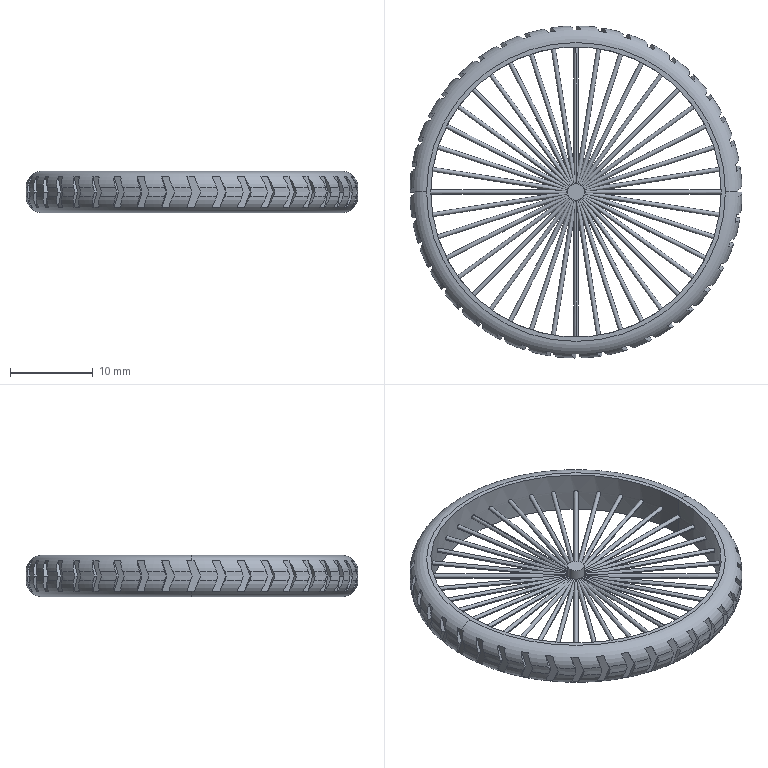Part | SolidWorks | features ICE 4, CirPattern 2, Fillet 2, Extrusion 1 | 1 solid | 338 faces | box 40 x 40 x 5 mm | volume 1342 mm3 | plane 204 | cylinder 128 | torus 4 | sphere 2 | commonest cylinder face diameters 0.5 x82 40 x40 2 x4 35 x2